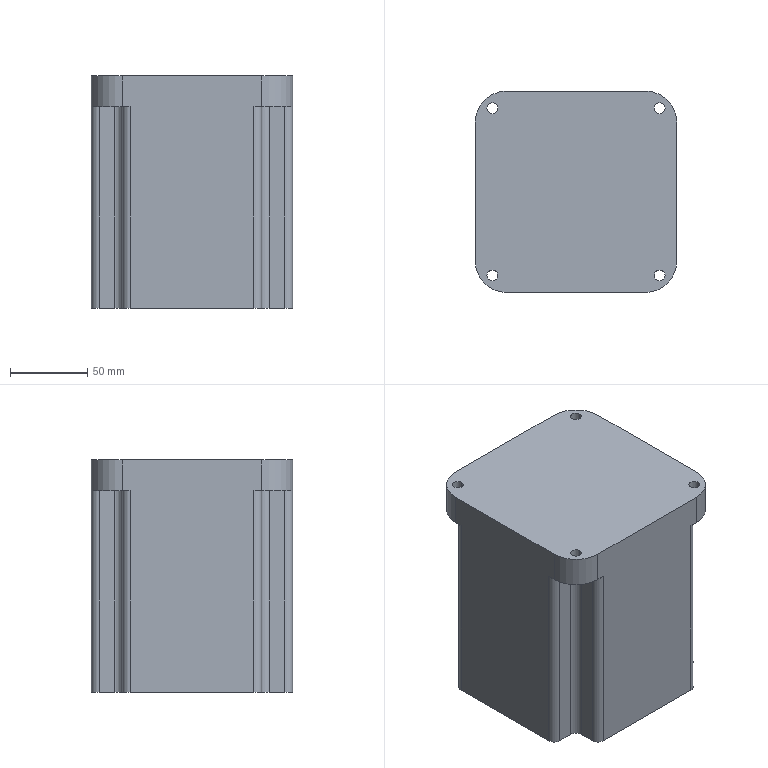Part | SolidWorks | features Fillet 3, CirPattern 2, ICE 2, Extrusion 1, RefAxis 1 | 1 solid | 42 faces | box 130 x 130 x 150 mm | volume 2314264 mm3 | cylinder 24 | plane 18 | commonest cylinder face diameters 10 x12 7 x8 40 x4
STEP:
#1=CARTESIAN_POINT('',(57.5,54.,150.));
#2=VERTEX_POINT('',#1);
#3=CARTESIAN_POINT('',(50.5,54.,150.));
#4=VERTEX_POINT('',#3);
#5=CARTESIAN_POINT('',(54.,54.,150.));
#6=DIRECTION('',(0.,0.,-1.));
#7=DIRECTION('',(-1.,0.,0.));
#8=AXIS2_PLACEMENT_3D('',#5,#6,#7);
#9=CIRCLE('',#8,3.5);
#10=EDGE_CURVE('',#2,#4,#9,.T.);
#11=ORIENTED_EDGE('',*,*,#10,.F.);
#12=CARTESIAN_POINT('',(57.5,54.,130.));
#13=VERTEX_POINT('',#12);
#14=CARTESIAN_POINT('',(57.5,54.,170.));
#15=DIRECTION('',(0.,0.,-1.));
#16=VECTOR('',#15,1000.);
#17=LINE('',#14,#16);
#18=EDGE_CURVE('',#2,#13,#17,.T.);
#19=ORIENTED_EDGE('',*,*,#18,.T.);
#20=CARTESIAN_POINT('',(50.5,54.,130.));
#21=VERTEX_POINT('',#20);
#22=CARTESIAN_POINT('',(54.,54.,130.));
#23=DIRECTION('',(0.,0.,-1.));
#24=DIRECTION('',(0.,1.,0.));
#25=AXIS2_PLACEMENT_3D('',#22,#23,#24);
#26=CIRCLE('',#25,3.5);
#27=EDGE_CURVE('',#13,#21,#26,.T.);
#28=ORIENTED_EDGE('',*,*,#27,.T.);
#29=CARTESIAN_POINT('',(50.5,54.,170.));
#30=DIRECTION('',(0.,0.,-1.));
#31=VECTOR('',#30,1000.);
#32=LINE('',#29,#31);
#33=EDGE_CURVE('',#4,#21,#32,.T.);
#34=ORIENTED_EDGE('',*,*,#33,.F.);
#35=EDGE_LOOP('',(#11,#19,#28,#34));
#36=FACE_OUTER_BOUND('',#35,.T.);
#37=CARTESIAN_POINT('',(54.,54.,170.));
#38=DIRECTION('',(0.,0.,-1.));
#39=DIRECTION('',(-1.,0.,0.));
#40=AXIS2_PLACEMENT_3D('',#37,#38,#39);
#41=CYLINDRICAL_SURFACE('',#40,3.5);
#42=ADVANCED_FACE('',(#36),#41,.F.);
#43=CARTESIAN_POINT('',(57.5,-54.,150.));
#44=VERTEX_POINT('',#43);
#45=CARTESIAN_POINT('',(50.5,-54.,150.));
#46=VERTEX_POINT('',#45);
#47=CARTESIAN_POINT('',(54.,-54.,150.));
#48=DIRECTION('',(0.,0.,-1.));
#49=DIRECTION('',(-1.,0.,0.));
#50=AXIS2_PLACEMENT_3D('',#47,#48,#49);
#51=CIRCLE('',#50,3.5);
#52=EDGE_CURVE('',#44,#46,#51,.T.);
#53=ORIENTED_EDGE('',*,*,#52,.F.);
#54=CARTESIAN_POINT('',(57.5,-54.,130.));
#55=VERTEX_POINT('',#54);
#56=CARTESIAN_POINT('',(57.5,-54.,170.));
#57=DIRECTION('',(0.,0.,-1.));
#58=VECTOR('',#57,1000.);
#59=LINE('',#56,#58);
#60=EDGE_CURVE('',#44,#55,#59,.T.);
#61=ORIENTED_EDGE('',*,*,#60,.T.);
#62=CARTESIAN_POINT('',(50.5,-54.,130.));
#63=VERTEX_POINT('',#62);
#64=CARTESIAN_POINT('',(54.,-54.,130.));
#65=DIRECTION('',(0.,0.,-1.));
#66=DIRECTION('',(1.,0.,0.));
#67=AXIS2_PLACEMENT_3D('',#64,#65,#66);
#68=CIRCLE('',#67,3.5);
#69=EDGE_CURVE('',#55,#63,#68,.T.);
#70=ORIENTED_EDGE('',*,*,#69,.T.);
#71=CARTESIAN_POINT('',(50.5,-54.,170.));
#72=DIRECTION('',(0.,0.,-1.));
#73=VECTOR('',#72,1000.);
#74=LINE('',#71,#73);
#75=EDGE_CURVE('',#46,#63,#74,.T.);
#76=ORIENTED_EDGE('',*,*,#75,.F.);
#77=EDGE_LOOP('',(#53,#61,#70,#76));
#78=FACE_OUTER_BOUND('',#77,.T.);
#79=CARTESIAN_POINT('',(54.,-54.,170.));
#80=DIRECTION('',(0.,0.,-1.));
#81=DIRECTION('',(-1.,0.,0.));
#82=AXIS2_PLACEMENT_3D('',#79,#80,#81);
#83=CYLINDRICAL_SURFACE('',#82,3.5);
#84=ADVANCED_FACE('',(#78),#83,.F.);
#85=CARTESIAN_POINT('',(-50.5,-54.,150.));
#86=VERTEX_POINT('',#85);
#87=CARTESIAN_POINT('',(-57.5,-54.,150.));
#88=VERTEX_POINT('',#87);
#89=CARTESIAN_POINT('',(-54.,-54.,150.));
#90=DIRECTION('',(0.,0.,-1.));
#91=DIRECTION('',(-1.,0.,0.));
#92=AXIS2_PLACEMENT_3D('',#89,#90,#91);
#93=CIRCLE('',#92,3.5);
#94=EDGE_CURVE('',#86,#88,#93,.T.);
#95=ORIENTED_EDGE('',*,*,#94,.F.);
#96=CARTESIAN_POINT('',(-50.5,-54.,130.));
#97=VERTEX_POINT('',#96);
#98=CARTESIAN_POINT('',(-50.5,-54.,170.));
#99=DIRECTION('',(0.,0.,-1.));
#100=VECTOR('',#99,1000.);
#101=LINE('',#98,#100);
#102=EDGE_CURVE('',#86,#97,#101,.T.);
#103=ORIENTED_EDGE('',*,*,#102,.T.);
#104=CARTESIAN_POINT('',(-57.5,-54.,130.));
#105=VERTEX_POINT('',#104);
#106=CARTESIAN_POINT('',(-54.,-54.,130.));
#107=DIRECTION('',(0.,0.,-1.));
#108=DIRECTION('',(0.,-1.,0.));
#109=AXIS2_PLACEMENT_3D('',#106,#107,#108);
#110=CIRCLE('',#109,3.5);
#111=EDGE_CURVE('',#97,#105,#110,.T.);
#112=ORIENTED_EDGE('',*,*,#111,.T.);
#113=CARTESIAN_POINT('',(-57.5,-54.,170.));
#114=DIRECTION('',(0.,0.,-1.));
#115=VECTOR('',#114,1000.);
#116=LINE('',#113,#115);
#117=EDGE_CURVE('',#88,#105,#116,.T.);
#118=ORIENTED_EDGE('',*,*,#117,.F.);
#119=EDGE_LOOP('',(#95,#103,#112,#118));
#120=FACE_OUTER_BOUND('',#119,.T.);
#121=CARTESIAN_POINT('',(-54.,-54.,170.));
#122=DIRECTION('',(0.,0.,-1.));
#123=DIRECTION('',(-1.,0.,0.));
#124=AXIS2_PLACEMENT_3D('',#121,#122,#123);
#125=CYLINDRICAL_SURFACE('',#124,3.5);
#126=ADVANCED_FACE('',(#120),#125,.F.);
#127=CARTESIAN_POINT('',(-50.5,54.,150.));
#128=VERTEX_POINT('',#127);
#129=CARTESIAN_POINT('',(-57.5,54.,150.));
#130=VERTEX_POINT('',#129);
#131=CARTESIAN_POINT('',(-54.,54.,150.));
#132=DIRECTION('',(0.,0.,-1.));
#133=DIRECTION('',(-1.,0.,0.));
#134=AXIS2_PLACEMENT_3D('',#131,#132,#133);
#135=CIRCLE('',#134,3.5);
#136=EDGE_CURVE('',#128,#130,#135,.T.);
#137=ORIENTED_EDGE('',*,*,#136,.F.);
#138=CARTESIAN_POINT('',(-50.5,54.,130.));
#139=VERTEX_POINT('',#138);
#140=CARTESIAN_POINT('',(-50.5,54.,170.));
#141=DIRECTION('',(0.,0.,-1.));
#142=VECTOR('',#141,1000.);
#143=LINE('',#140,#142);
#144=EDGE_CURVE('',#128,#139,#143,.T.);
#145=ORIENTED_EDGE('',*,*,#144,.T.);
#146=CARTESIAN_POINT('',(-57.5,54.,130.));
#147=VERTEX_POINT('',#146);
#148=CARTESIAN_POINT('',(-54.,54.,130.));
#149=DIRECTION('',(0.,0.,-1.));
#150=DIRECTION('',(-1.,0.,0.));
#151=AXIS2_PLACEMENT_3D('',#148,#149,#150);
#152=CIRCLE('',#151,3.5);
#153=EDGE_CURVE('',#139,#147,#152,.T.);
#154=ORIENTED_EDGE('',*,*,#153,.T.);
#155=CARTESIAN_POINT('',(-57.5,54.,170.));
#156=DIRECTION('',(0.,0.,-1.));
#157=VECTOR('',#156,1000.);
#158=LINE('',#155,#157);
#159=EDGE_CURVE('',#130,#147,#158,.T.);
#160=ORIENTED_EDGE('',*,*,#159,.F.);
#161=EDGE_LOOP('',(#137,#145,#154,#160));
#162=FACE_OUTER_BOUND('',#161,.T.);
#163=CARTESIAN_POINT('',(-54.,54.,170.));
#164=DIRECTION('',(0.,0.,-1.));
#165=DIRECTION('',(-1.,0.,0.));
#166=AXIS2_PLACEMENT_3D('',#163,#164,#165);
#167=CYLINDRICAL_SURFACE('',#166,3.5);
#168=ADVANCED_FACE('',(#162),#167,.F.);
#169=CARTESIAN_POINT('',(-65.,-45.,130.));
#170=VERTEX_POINT('',#169);
#171=CARTESIAN_POINT('',(-65.,-45.,150.));
#172=VERTEX_POINT('',#171);
#173=CARTESIAN_POINT('',(-65.,-45.,150.));
#174=DIRECTION('',(0.,0.,1.));
#175=VECTOR('',#174,1000.);
#176=LINE('',#173,#175);
#177=EDGE_CURVE('',#170,#172,#176,.T.);
#178=ORIENTED_EDGE('',*,*,#177,.F.);
#179=CARTESIAN_POINT('',(-45.,-65.,130.));
#180=VERTEX_POINT('',#179);
#181=CARTESIAN_POINT('',(-45.,-45.,130.));
#182=DIRECTION('',(0.,0.,1.));
#183=DIRECTION('',(-1.,0.,0.));
#184=AXIS2_PLACEMENT_3D('',#181,#182,#183);
#185=CIRCLE('',#184,20.);
#186=EDGE_CURVE('',#170,#180,#185,.T.);
#187=ORIENTED_EDGE('',*,*,#186,.T.);
#188=CARTESIAN_POINT('',(-45.,-65.,150.));
#189=VERTEX_POINT('',#188);
#190=CARTESIAN_POINT('',(-45.,-65.,150.));
#191=DIRECTION('',(0.,0.,-1.));
#192=VECTOR('',#191,1000.);
#193=LINE('',#190,#192);
#194=EDGE_CURVE('',#189,#180,#193,.T.);
#195=ORIENTED_EDGE('',*,*,#194,.F.);
#196=CARTESIAN_POINT('',(-45.,-45.,150.));
#197=DIRECTION('',(0.,0.,1.));
#198=DIRECTION('',(-1.,0.,0.));
#199=AXIS2_PLACEMENT_3D('',#196,#197,#198);
#200=CIRCLE('',#199,20.);
#201=EDGE_CURVE('',#172,#189,#200,.T.);
#202=ORIENTED_EDGE('',*,*,#201,.F.);
#203=EDGE_LOOP('',(#178,#187,#195,#202));
#204=FACE_OUTER_BOUND('',#203,.T.);
#205=CARTESIAN_POINT('',(-45.,-45.,150.));
#206=DIRECTION('',(0.,0.,-1.));
#207=DIRECTION('',(-1.,0.,0.));
#208=AXIS2_PLACEMENT_3D('',#205,#206,#207);
#209=CYLINDRICAL_SURFACE('',#208,20.);
#210=ADVANCED_FACE('',(#204),#209,.T.);
#211=CARTESIAN_POINT('',(45.,-65.,130.));
#212=VERTEX_POINT('',#211);
#213=CARTESIAN_POINT('',(45.,-65.,150.));
#214=VERTEX_POINT('',#213);
#215=CARTESIAN_POINT('',(45.,-65.,150.));
#216=DIRECTION('',(0.,0.,1.));
#217=VECTOR('',#216,1000.);
#218=LINE('',#215,#217);
#219=EDGE_CURVE('',#212,#214,#218,.T.);
#220=ORIENTED_EDGE('',*,*,#219,.F.);
#221=CARTESIAN_POINT('',(65.,-45.,130.));
#222=VERTEX_POINT('',#221);
#223=CARTESIAN_POINT('',(45.,-45.,130.));
#224=DIRECTION('',(0.,0.,1.));
#225=DIRECTION('',(-1.,0.,0.));
#226=AXIS2_PLACEMENT_3D('',#223,#224,#225);
#227=CIRCLE('',#226,20.);
#228=EDGE_CURVE('',#212,#222,#227,.T.);
#229=ORIENTED_EDGE('',*,*,#228,.T.);
#230=CARTESIAN_POINT('',(65.,-45.,150.));
#231=VERTEX_POINT('',#230);
#232=CARTESIAN_POINT('',(65.,-45.,150.));
#233=DIRECTION('',(0.,0.,-1.));
#234=VECTOR('',#233,1000.);
#235=LINE('',#232,#234);
#236=EDGE_CURVE('',#231,#222,#235,.T.);
#237=ORIENTED_EDGE('',*,*,#236,.F.);
#238=CARTESIAN_POINT('',(45.,-45.,150.));
#239=DIRECTION('',(0.,0.,1.));
#240=DIRECTION('',(-1.,0.,0.));
#241=AXIS2_PLACEMENT_3D('',#238,#239,#240);
#242=CIRCLE('',#241,20.);
#243=EDGE_CURVE('',#214,#231,#242,.T.);
#244=ORIENTED_EDGE('',*,*,#243,.F.);
#245=EDGE_LOOP('',(#220,#229,#237,#244));
#246=FACE_OUTER_BOUND('',#245,.T.);
#247=CARTESIAN_POINT('',(45.,-45.,150.));
#248=DIRECTION('',(0.,0.,-1.));
#249=DIRECTION('',(-1.,0.,0.));
#250=AXIS2_PLACEMENT_3D('',#247,#248,#249);
#251=CYLINDRICAL_SURFACE('',#250,20.);
#252=ADVANCED_FACE('',(#246),#251,.T.);
#253=CARTESIAN_POINT('',(-45.,65.,130.));
#254=VERTEX_POINT('',#253);
#255=CARTESIAN_POINT('',(-45.,65.,150.));
#256=VERTEX_POINT('',#255);
#257=CARTESIAN_POINT('',(-45.,65.,150.));
#258=DIRECTION('',(0.,0.,1.));
#259=VECTOR('',#258,1000.);
#260=LINE('',#257,#259);
#261=EDGE_CURVE('',#254,#256,#260,.T.);
#262=ORIENTED_EDGE('',*,*,#261,.F.);
#263=CARTESIAN_POINT('',(-65.,45.,130.));
#264=VERTEX_POINT('',#263);
#265=CARTESIAN_POINT('',(-45.,45.,130.));
#266=DIRECTION('',(0.,0.,1.));
#267=DIRECTION('',(-1.,0.,0.));
#268=AXIS2_PLACEMENT_3D('',#265,#266,#267);
#269=CIRCLE('',#268,20.);
#270=EDGE_CURVE('',#254,#264,#269,.T.);
#271=ORIENTED_EDGE('',*,*,#270,.T.);
#272=CARTESIAN_POINT('',(-65.,45.,150.));
#273=VERTEX_POINT('',#272);
#274=CARTESIAN_POINT('',(-65.,45.,150.));
#275=DIRECTION('',(0.,0.,-1.));
#276=VECTOR('',#275,1000.);
#277=LINE('',#274,#276);
#278=EDGE_CURVE('',#273,#264,#277,.T.);
#279=ORIENTED_EDGE('',*,*,#278,.F.);
#280=CARTESIAN_POINT('',(-45.,45.,150.));
#281=DIRECTION('',(0.,0.,1.));
#282=DIRECTION('',(-1.,0.,0.));
#283=AXIS2_PLACEMENT_3D('',#280,#281,#282);
#284=CIRCLE('',#283,20.);
#285=EDGE_CURVE('',#256,#273,#284,.T.);
#286=ORIENTED_EDGE('',*,*,#285,.F.);
#287=EDGE_LOOP('',(#262,#271,#279,#286));
#288=FACE_OUTER_BOUND('',#287,.T.);
#289=CARTESIAN_POINT('',(-45.,45.,150.));
#290=DIRECTION('',(0.,0.,-1.));
#291=DIRECTION('',(-1.,0.,0.));
#292=AXIS2_PLACEMENT_3D('',#289,#290,#291);
#293=CYLINDRICAL_SURFACE('',#292,20.);
#294=ADVANCED_FACE('',(#288),#293,.T.);
#295=CARTESIAN_POINT('',(65.,45.,130.));
#296=VERTEX_POINT('',#295);
#297=CARTESIAN_POINT('',(65.,45.,150.));
#298=VERTEX_POINT('',#297);
#299=CARTESIAN_POINT('',(65.,45.,150.));
#300=DIRECTION('',(0.,0.,1.));
#301=VECTOR('',#300,1000.);
#302=LINE('',#299,#301);
#303=EDGE_CURVE('',#296,#298,#302,.T.);
#304=ORIENTED_EDGE('',*,*,#303,.F.);
#305=CARTESIAN_POINT('',(45.,65.,130.));
#306=VERTEX_POINT('',#305);
#307=CARTESIAN_POINT('',(45.,45.,130.));
#308=DIRECTION('',(0.,0.,1.));
#309=DIRECTION('',(-1.,0.,0.));
#310=AXIS2_PLACEMENT_3D('',#307,#308,#309);
#311=CIRCLE('',#310,20.);
#312=EDGE_CURVE('',#296,#306,#311,.T.);
#313=ORIENTED_EDGE('',*,*,#312,.T.);
#314=CARTESIAN_POINT('',(45.,65.,150.));
#315=VERTEX_POINT('',#314);
#316=CARTESIAN_POINT('',(45.,65.,150.));
#317=DIRECTION('',(0.,0.,-1.));
#318=VECTOR('',#317,1000.);
#319=LINE('',#316,#318);
#320=EDGE_CURVE('',#315,#306,#319,.T.);
#321=ORIENTED_EDGE('',*,*,#320,.F.);
#322=CARTESIAN_POINT('',(45.,45.,150.));
#323=DIRECTION('',(0.,0.,1.));
#324=DIRECTION('',(-1.,0.,0.));
#325=AXIS2_PLACEMENT_3D('',#322,#323,#324);
#326=CIRCLE('',#325,20.);
#327=EDGE_CURVE('',#298,#315,#326,.T.);
#328=ORIENTED_EDGE('',*,*,#327,.F.);
#329=EDGE_LOOP('',(#304,#313,#321,#328));
#330=FACE_OUTER_BOUND('',#329,.T.);
#331=CARTESIAN_POINT('',(45.,45.,150.));
#332=DIRECTION('',(0.,0.,-1.));
#333=DIRECTION('',(-1.,0.,0.));
#334=AXIS2_PLACEMENT_3D('',#331,#332,#333);
#335=CYLINDRICAL_SURFACE('',#334,20.);
#336=ADVANCED_FACE('',(#330),#335,.T.);
#337=CARTESIAN_POINT('',(65.,-40.,0.));
#338=VERTEX_POINT('',#337);
#339=CARTESIAN_POINT('',(65.,40.,0.));
#340=VERTEX_POINT('',#339);
#341=CARTESIAN_POINT('',(65.,-65.,0.));
#342=DIRECTION('',(0.,1.,0.));
#343=VECTOR('',#342,1000.);
#344=LINE('',#341,#343);
#345=EDGE_CURVE('',#338,#340,#344,.T.);
#346=ORIENTED_EDGE('',*,*,#345,.T.);
#347=CARTESIAN_POINT('',(65.,40.,130.));
#348=VERTEX_POINT('',#347);
#349=CARTESIAN_POINT('',(65.,40.,150.));
#350=DIRECTION('',(0.,0.,1.));
#351=VECTOR('',#350,1000.);
#352=LINE('',#349,#351);
#353=EDGE_CURVE('',#340,#348,#352,.T.);
#354=ORIENTED_EDGE('',*,*,#353,.T.);
#355=CARTESIAN_POINT('',(65.,0.,130.));
#356=DIRECTION('',(0.,1.,0.));
#357=VECTOR('',#356,1000.);
#358=LINE('',#355,#357);
#359=EDGE_CURVE('',#348,#296,#358,.T.);
#360=ORIENTED_EDGE('',*,*,#359,.T.);
#361=ORIENTED_EDGE('',*,*,#303,.T.);
#362=CARTESIAN_POINT('',(65.,-65.,150.));
#363=DIRECTION('',(0.,1.,0.));
#364=VECTOR('',#363,1000.);
#365=LINE('',#362,#364);
#366=EDGE_CURVE('',#231,#298,#365,.T.);
#367=ORIENTED_EDGE('',*,*,#366,.F.);
#368=ORIENTED_EDGE('',*,*,#236,.T.);
#369=CARTESIAN_POINT('',(65.,-40.,130.));
#370=VERTEX_POINT('',#369);
#371=CARTESIAN_POINT('',(65.,0.,130.));
#372=DIRECTION('',(0.,1.,0.));
#373=VECTOR('',#372,1000.);
#374=LINE('',#371,#373);
#375=EDGE_CURVE('',#222,#370,#374,.T.);
#376=ORIENTED_EDGE('',*,*,#375,.T.);
#377=CARTESIAN_POINT('',(65.,-40.,150.));
#378=DIRECTION('',(0.,0.,-1.));
#379=VECTOR('',#378,1000.);
#380=LINE('',#377,#379);
#381=EDGE_CURVE('',#370,#338,#380,.T.);
#382=ORIENTED_EDGE('',*,*,#381,.T.);
#383=EDGE_LOOP('',(#346,#354,#360,#361,#367,#368,#376,#382));
#384=FACE_OUTER_BOUND('',#383,.T.);
#385=CARTESIAN_POINT('',(65.,-65.,150.));
#386=DIRECTION('',(-1.,0.,0.));
#387=DIRECTION('',(0.,0.,1.));
#388=AXIS2_PLACEMENT_3D('',#385,#386,#387);
#389=PLANE('',#388);
#390=ADVANCED_FACE('',(#384),#389,.F.);
#391=CARTESIAN_POINT('',(40.,65.,130.));
#392=VERTEX_POINT('',#391);
#393=CARTESIAN_POINT('',(0.,65.,130.));
#394=DIRECTION('',(-1.,0.,0.));
#395=VECTOR('',#394,1000.);
#396=LINE('',#393,#395);
#397=EDGE_CURVE('',#306,#392,#396,.T.);
#398=ORIENTED_EDGE('',*,*,#397,.T.);
#399=CARTESIAN_POINT('',(40.,65.,0.));
#400=VERTEX_POINT('',#399);
#401=CARTESIAN_POINT('',(40.,65.,150.));
#402=DIRECTION('',(0.,0.,-1.));
#403=VECTOR('',#402,1000.);
#404=LINE('',#401,#403);
#405=EDGE_CURVE('',#392,#400,#404,.T.);
#406=ORIENTED_EDGE('',*,*,#405,.T.);
#407=CARTESIAN_POINT('',(-40.,65.,0.));
#408=VERTEX_POINT('',#407);
#409=CARTESIAN_POINT('',(-65.,65.,0.));
#410=DIRECTION('',(-1.,0.,0.));
#411=VECTOR('',#410,1000.);
#412=LINE('',#409,#411);
#413=EDGE_CURVE('',#400,#408,#412,.T.);
#414=ORIENTED_EDGE('',*,*,#413,.T.);
#415=CARTESIAN_POINT('',(-40.,65.,130.));
#416=VERTEX_POINT('',#415);
#417=CARTESIAN_POINT('',(-40.,65.,150.));
#418=DIRECTION('',(0.,0.,1.));
#419=VECTOR('',#418,1000.);
#420=LINE('',#417,#419);
#421=EDGE_CURVE('',#408,#416,#420,.T.);
#422=ORIENTED_EDGE('',*,*,#421,.T.);
#423=CARTESIAN_POINT('',(0.,65.,130.));
#424=DIRECTION('',(-1.,0.,0.));
#425=VECTOR('',#424,1000.);
#426=LINE('',#423,#425);
#427=EDGE_CURVE('',#416,#254,#426,.T.);
#428=ORIENTED_EDGE('',*,*,#427,.T.);
#429=ORIENTED_EDGE('',*,*,#261,.T.);
#430=CARTESIAN_POINT('',(-65.,65.,150.));
#431=DIRECTION('',(-1.,0.,0.));
#432=VECTOR('',#431,1000.);
#433=LINE('',#430,#432);
#434=EDGE_CURVE('',#315,#256,#433,.T.);
#435=ORIENTED_EDGE('',*,*,#434,.F.);
#436=ORIENTED_EDGE('',*,*,#320,.T.);
#437=EDGE_LOOP('',(#398,#406,#414,#422,#428,#429,#435,#436));
#438=FACE_OUTER_BOUND('',#437,.T.);
#439=CARTESIAN_POINT('',(-65.,65.,150.));
#440=DIRECTION('',(0.,-1.,0.));
#441=DIRECTION('',(0.,0.,-1.));
#442=AXIS2_PLACEMENT_3D('',#439,#440,#441);
#443=PLANE('',#442);
#444=ADVANCED_FACE('',(#438),#443,.F.);
#445=CARTESIAN_POINT('',(-65.,40.,130.));
#446=VERTEX_POINT('',#445);
#447=CARTESIAN_POINT('',(-65.,0.,130.));
#448=DIRECTION('',(0.,-1.,0.));
#449=VECTOR('',#448,1000.);
#450=LINE('',#447,#449);
#451=EDGE_CURVE('',#264,#446,#450,.T.);
#452=ORIENTED_EDGE('',*,*,#451,.T.);
#453=CARTESIAN_POINT('',(-65.,40.,0.));
#454=VERTEX_POINT('',#453);
#455=CARTESIAN_POINT('',(-65.,40.,150.));
#456=DIRECTION('',(0.,0.,-1.));
#457=VECTOR('',#456,1000.);
#458=LINE('',#455,#457);
#459=EDGE_CURVE('',#446,#454,#458,.T.);
#460=ORIENTED_EDGE('',*,*,#459,.T.);
#461=CARTESIAN_POINT('',(-65.,-40.,0.));
#462=VERTEX_POINT('',#461);
#463=CARTESIAN_POINT('',(-65.,-65.,0.));
#464=DIRECTION('',(0.,-1.,0.));
#465=VECTOR('',#464,1000.);
#466=LINE('',#463,#465);
#467=EDGE_CURVE('',#454,#462,#466,.T.);
#468=ORIENTED_EDGE('',*,*,#467,.T.);
#469=CARTESIAN_POINT('',(-65.,-40.,130.));
#470=VERTEX_POINT('',#469);
#471=CARTESIAN_POINT('',(-65.,-40.,150.));
#472=DIRECTION('',(0.,0.,1.));
#473=VECTOR('',#472,1000.);
#474=LINE('',#471,#473);
#475=EDGE_CURVE('',#462,#470,#474,.T.);
#476=ORIENTED_EDGE('',*,*,#475,.T.);
#477=CARTESIAN_POINT('',(-65.,0.,130.));
#478=DIRECTION('',(0.,-1.,0.));
#479=VECTOR('',#478,1000.);
#480=LINE('',#477,#479);
#481=EDGE_CURVE('',#470,#170,#480,.T.);
#482=ORIENTED_EDGE('',*,*,#481,.T.);
#483=ORIENTED_EDGE('',*,*,#177,.T.);
#484=CARTESIAN_POINT('',(-65.,-65.,150.));
#485=DIRECTION('',(0.,-1.,0.));
#486=VECTOR('',#485,1000.);
#487=LINE('',#484,#486);
#488=EDGE_CURVE('',#273,#172,#487,.T.);
#489=ORIENTED_EDGE('',*,*,#488,.F.);
#490=ORIENTED_EDGE('',*,*,#278,.T.);
#491=EDGE_LOOP('',(#452,#460,#468,#476,#482,#483,#489,#490));
#492=FACE_OUTER_BOUND('',#491,.T.);
#493=CARTESIAN_POINT('',(-65.,-65.,150.));
#494=DIRECTION('',(1.,0.,0.));
#495=DIRECTION('',(0.,0.,-1.));
#496=AXIS2_PLACEMENT_3D('',#493,#494,#495);
#497=PLANE('',#496);
#498=ADVANCED_FACE('',(#492),#497,.F.);
#499=CARTESIAN_POINT('',(-40.,-65.,130.));
#500=VERTEX_POINT('',#499);
#501=CARTESIAN_POINT('',(0.,-65.,130.));
#502=DIRECTION('',(1.,0.,0.));
#503=VECTOR('',#502,1000.);
#504=LINE('',#501,#503);
#505=EDGE_CURVE('',#180,#500,#504,.T.);
#506=ORIENTED_EDGE('',*,*,#505,.T.);
#507=CARTESIAN_POINT('',(-40.,-65.,0.));
#508=VERTEX_POINT('',#507);
#509=CARTESIAN_POINT('',(-40.,-65.,150.));
#510=DIRECTION('',(0.,0.,-1.));
#511=VECTOR('',#510,1000.);
#512=LINE('',#509,#511);
#513=EDGE_CURVE('',#500,#508,#512,.T.);
#514=ORIENTED_EDGE('',*,*,#513,.T.);
#515=CARTESIAN_POINT('',(40.,-65.,0.));
#516=VERTEX_POINT('',#515);
#517=CARTESIAN_POINT('',(-65.,-65.,0.));
#518=DIRECTION('',(1.,0.,0.));
#519=VECTOR('',#518,1000.);
#520=LINE('',#517,#519);
#521=EDGE_CURVE('',#508,#516,#520,.T.);
#522=ORIENTED_EDGE('',*,*,#521,.T.);
#523=CARTESIAN_POINT('',(40.,-65.,130.));
#524=VERTEX_POINT('',#523);
#525=CARTESIAN_POINT('',(40.,-65.,150.));
#526=DIRECTION('',(0.,0.,1.));
#527=VECTOR('',#526,1000.);
#528=LINE('',#525,#527);
#529=EDGE_CURVE('',#516,#524,#528,.T.);
#530=ORIENTED_EDGE('',*,*,#529,.T.);
#531=CARTESIAN_POINT('',(0.,-65.,130.));
#532=DIRECTION('',(1.,0.,0.));
#533=VECTOR('',#532,1000.);
#534=LINE('',#531,#533);
#535=EDGE_CURVE('',#524,#212,#534,.T.);
#536=ORIENTED_EDGE('',*,*,#535,.T.);
#537=ORIENTED_EDGE('',*,*,#219,.T.);
#538=CARTESIAN_POINT('',(-65.,-65.,150.));
#539=DIRECTION('',(1.,0.,0.));
#540=VECTOR('',#539,1000.);
#541=LINE('',#538,#540);
#542=EDGE_CURVE('',#189,#214,#541,.T.);
#543=ORIENTED_EDGE('',*,*,#542,.F.);
#544=ORIENTED_EDGE('',*,*,#194,.T.);
#545=EDGE_LOOP('',(#506,#514,#522,#530,#536,#537,#543,#544));
#546=FACE_OUTER_BOUND('',#545,.T.);
#547=CARTESIAN_POINT('',(-65.,-65.,150.));
#548=DIRECTION('',(0.,1.,0.));
#549=DIRECTION('',(0.,0.,1.));
#550=AXIS2_PLACEMENT_3D('',#547,#548,#549);
#551=PLANE('',#550);
#552=ADVANCED_FACE('',(#546),#551,.F.);
#553=CARTESIAN_POINT('',(-54.,-54.,150.));
#554=DIRECTION('',(0.,0.,-1.));
#555=DIRECTION('',(-1.,0.,0.));
#556=AXIS2_PLACEMENT_3D('',#553,#554,#555);
#557=CIRCLE('',#556,3.5);
#558=EDGE_CURVE('',#88,#86,#557,.T.);
#559=ORIENTED_EDGE('',*,*,#558,.T.);
#560=ORIENTED_EDGE('',*,*,#94,.T.);
#561=EDGE_LOOP('',(#559,#560));
#562=FACE_BOUND('',#561,.T.);
#563=CARTESIAN_POINT('',(54.,-54.,150.));
#564=DIRECTION('',(0.,0.,-1.));
#565=DIRECTION('',(-1.,0.,0.));
#566=AXIS2_PLACEMENT_3D('',#563,#564,#565);
#567=CIRCLE('',#566,3.5);
#568=EDGE_CURVE('',#46,#44,#567,.T.);
#569=ORIENTED_EDGE('',*,*,#568,.T.);
#570=ORIENTED_EDGE('',*,*,#52,.T.);
#571=EDGE_LOOP('',(#569,#570));
#572=FACE_BOUND('',#571,.T.);
#573=CARTESIAN_POINT('',(54.,54.,150.));
#574=DIRECTION('',(0.,0.,-1.));
#575=DIRECTION('',(-1.,0.,0.));
#576=AXIS2_PLACEMENT_3D('',#573,#574,#575);
#577=CIRCLE('',#576,3.5);
#578=EDGE_CURVE('',#4,#2,#577,.T.);
#579=ORIENTED_EDGE('',*,*,#578,.T.);
#580=ORIENTED_EDGE('',*,*,#10,.T.);
#581=EDGE_LOOP('',(#579,#580));
#582=FACE_BOUND('',#581,.T.);
#583=CARTESIAN_POINT('',(-54.,54.,150.));
#584=DIRECTION('',(0.,0.,-1.));
#585=DIRECTION('',(-1.,0.,0.));
#586=AXIS2_PLACEMENT_3D('',#583,#584,#585);
#587=CIRCLE('',#586,3.5);
#588=EDGE_CURVE('',#130,#128,#587,.T.);
#589=ORIENTED_EDGE('',*,*,#588,.T.);
#590=ORIENTED_EDGE('',*,*,#136,.T.);
#591=EDGE_LOOP('',(#589,#590));
#592=FACE_BOUND('',#591,.T.);
#593=ORIENTED_EDGE('',*,*,#488,.T.);
#594=ORIENTED_EDGE('',*,*,#201,.T.);
#595=ORIENTED_EDGE('',*,*,#542,.T.);
#596=ORIENTED_EDGE('',*,*,#243,.T.);
#597=ORIENTED_EDGE('',*,*,#366,.T.);
#598=ORIENTED_EDGE('',*,*,#327,.T.);
#599=ORIENTED_EDGE('',*,*,#434,.T.);
#600=ORIENTED_EDGE('',*,*,#285,.T.);
#601=EDGE_LOOP('',(#593,#594,#595,#596,#597,#598,#599,#600));
#602=FACE_OUTER_BOUND('',#601,.T.);
#603=CARTESIAN_POINT('',(0.,0.,150.));
#604=DIRECTION('',(0.,0.,-1.));
#605=DIRECTION('',(-1.,0.,0.));
#606=AXIS2_PLACEMENT_3D('',#603,#604,#605);
#607=PLANE('',#606);
#608=ADVANCED_FACE('',(#562,#572,#582,#592,#602),#607,.F.);
#609=CARTESIAN_POINT('',(60.,45.,0.));
#610=VERTEX_POINT('',#609);
#611=CARTESIAN_POINT('',(50.,45.,0.));
#612=VERTEX_POINT('',#611);
#613=CARTESIAN_POINT('',(114.063,45.,0.));
#614=DIRECTION('',(-1.,0.,0.));
#615=VECTOR('',#614,1000.);
#616=LINE('',#613,#615);
#617=EDGE_CURVE('',#610,#612,#616,.T.);
#618=ORIENTED_EDGE('',*,*,#617,.F.);
#619=CARTESIAN_POINT('',(60.,40.,0.));
#620=DIRECTION('',(0.,0.,-1.));
#621=DIRECTION('',(-1.,0.,0.));
#622=AXIS2_PLACEMENT_3D('',#619,#620,#621);
#623=CIRCLE('',#622,5.);
#624=EDGE_CURVE('',#610,#340,#623,.T.);
#625=ORIENTED_EDGE('',*,*,#624,.T.);
#626=ORIENTED_EDGE('',*,*,#345,.F.);
#627=CARTESIAN_POINT('',(60.,-45.,0.));
#628=VERTEX_POINT('',#627);
#629=CARTESIAN_POINT('',(60.,-40.,0.));
#630=DIRECTION('',(0.,0.,-1.));
#631=DIRECTION('',(-1.,0.,0.));
#632=AXIS2_PLACEMENT_3D('',#629,#630,#631);
#633=CIRCLE('',#632,5.);
#634=EDGE_CURVE('',#338,#628,#633,.T.);
#635=ORIENTED_EDGE('',*,*,#634,.T.);
#636=CARTESIAN_POINT('',(50.,-45.,0.));
#637=VERTEX_POINT('',#636);
#638=CARTESIAN_POINT('',(130.712,-45.,0.));
#639=DIRECTION('',(1.,0.,0.));
#640=VECTOR('',#639,1000.);
#641=LINE('',#638,#640);
#642=EDGE_CURVE('',#637,#628,#641,.T.);
#643=ORIENTED_EDGE('',*,*,#642,.F.);
#644=CARTESIAN_POINT('',(45.,-50.,0.));
#645=VERTEX_POINT('',#644);
#646=CARTESIAN_POINT('',(50.,-50.,0.));
#647=DIRECTION('',(0.,0.,1.));
#648=DIRECTION('',(-1.,0.,0.));
#649=AXIS2_PLACEMENT_3D('',#646,#647,#648);
#650=CIRCLE('',#649,5.);
#651=EDGE_CURVE('',#637,#645,#650,.T.);
#652=ORIENTED_EDGE('',*,*,#651,.T.);
#653=CARTESIAN_POINT('',(45.,-60.,0.));
#654=VERTEX_POINT('',#653);
#655=CARTESIAN_POINT('',(45.,-114.063,0.));
#656=DIRECTION('',(0.,1.,0.));
#657=VECTOR('',#656,1000.);
#658=LINE('',#655,#657);
#659=EDGE_CURVE('',#654,#645,#658,.T.);
#660=ORIENTED_EDGE('',*,*,#659,.F.);
#661=CARTESIAN_POINT('',(40.,-60.,0.));
#662=DIRECTION('',(0.,0.,-1.));
#663=DIRECTION('',(-1.,0.,0.));
#664=AXIS2_PLACEMENT_3D('',#661,#662,#663);
#665=CIRCLE('',#664,5.);
#666=EDGE_CURVE('',#654,#516,#665,.T.);
#667=ORIENTED_EDGE('',*,*,#666,.T.);
#668=ORIENTED_EDGE('',*,*,#521,.F.);
#669=CARTESIAN_POINT('',(-45.,-60.,0.));
#670=VERTEX_POINT('',#669);
#671=CARTESIAN_POINT('',(-40.,-60.,0.));
#672=DIRECTION('',(0.,0.,-1.));
#673=DIRECTION('',(-1.,0.,0.));
#674=AXIS2_PLACEMENT_3D('',#671,#672,#673);
#675=CIRCLE('',#674,5.);
#676=EDGE_CURVE('',#508,#670,#675,.T.);
#677=ORIENTED_EDGE('',*,*,#676,.T.);
#678=CARTESIAN_POINT('',(-45.,-50.,0.));
#679=VERTEX_POINT('',#678);
#680=CARTESIAN_POINT('',(-45.,-130.712,0.));
#681=DIRECTION('',(0.,-1.,0.));
#682=VECTOR('',#681,1000.);
#683=LINE('',#680,#682);
#684=EDGE_CURVE('',#679,#670,#683,.T.);
#685=ORIENTED_EDGE('',*,*,#684,.F.);
#686=CARTESIAN_POINT('',(-50.,-45.,0.));
#687=VERTEX_POINT('',#686);
#688=CARTESIAN_POINT('',(-50.,-50.,0.));
#689=DIRECTION('',(0.,0.,1.));
#690=DIRECTION('',(-1.,0.,0.));
#691=AXIS2_PLACEMENT_3D('',#688,#689,#690);
#692=CIRCLE('',#691,5.);
#693=EDGE_CURVE('',#679,#687,#692,.T.);
#694=ORIENTED_EDGE('',*,*,#693,.T.);
#695=CARTESIAN_POINT('',(-60.,-45.,0.));
#696=VERTEX_POINT('',#695);
#697=CARTESIAN_POINT('',(-114.063,-45.,0.));
#698=DIRECTION('',(1.,0.,0.));
#699=VECTOR('',#698,1000.);
#700=LINE('',#697,#699);
#701=EDGE_CURVE('',#696,#687,#700,.T.);
#702=ORIENTED_EDGE('',*,*,#701,.F.);
#703=CARTESIAN_POINT('',(-60.,-40.,0.));
#704=DIRECTION('',(0.,0.,-1.));
#705=DIRECTION('',(-1.,0.,0.));
#706=AXIS2_PLACEMENT_3D('',#703,#704,#705);
#707=CIRCLE('',#706,5.);
#708=EDGE_CURVE('',#696,#462,#707,.T.);
#709=ORIENTED_EDGE('',*,*,#708,.T.);
#710=ORIENTED_EDGE('',*,*,#467,.F.);
#711=CARTESIAN_POINT('',(-60.,45.,0.));
#712=VERTEX_POINT('',#711);
#713=CARTESIAN_POINT('',(-60.,40.,0.));
#714=DIRECTION('',(0.,0.,-1.));
#715=DIRECTION('',(-1.,0.,0.));
#716=AXIS2_PLACEMENT_3D('',#713,#714,#715);
#717=CIRCLE('',#716,5.);
#718=EDGE_CURVE('',#454,#712,#717,.T.);
#719=ORIENTED_EDGE('',*,*,#718,.T.);
#720=CARTESIAN_POINT('',(-50.,45.,0.));
#721=VERTEX_POINT('',#720);
#722=CARTESIAN_POINT('',(-130.712,45.,0.));
#723=DIRECTION('',(-1.,0.,0.));
#724=VECTOR('',#723,1000.);
#725=LINE('',#722,#724);
#726=EDGE_CURVE('',#721,#712,#725,.T.);
#727=ORIENTED_EDGE('',*,*,#726,.F.);
#728=CARTESIAN_POINT('',(-45.,50.,0.));
#729=VERTEX_POINT('',#728);
#730=CARTESIAN_POINT('',(-50.,50.,0.));
#731=DIRECTION('',(0.,0.,1.));
#732=DIRECTION('',(-1.,0.,0.));
#733=AXIS2_PLACEMENT_3D('',#730,#731,#732);
#734=CIRCLE('',#733,5.);
#735=EDGE_CURVE('',#721,#729,#734,.T.);
#736=ORIENTED_EDGE('',*,*,#735,.T.);
#737=CARTESIAN_POINT('',(-45.,60.,0.));
#738=VERTEX_POINT('',#737);
#739=CARTESIAN_POINT('',(-45.,114.063,0.));
#740=DIRECTION('',(0.,-1.,0.));
#741=VECTOR('',#740,1000.);
#742=LINE('',#739,#741);
#743=EDGE_CURVE('',#738,#729,#742,.T.);
#744=ORIENTED_EDGE('',*,*,#743,.F.);
#745=CARTESIAN_POINT('',(-40.,60.,0.));
#746=DIRECTION('',(0.,0.,-1.));
#747=DIRECTION('',(-1.,0.,0.));
#748=AXIS2_PLACEMENT_3D('',#745,#746,#747);
#749=CIRCLE('',#748,5.);
#750=EDGE_CURVE('',#738,#408,#749,.T.);
#751=ORIENTED_EDGE('',*,*,#750,.T.);
#752=ORIENTED_EDGE('',*,*,#413,.F.);
#753=CARTESIAN_POINT('',(45.,60.,0.));
#754=VERTEX_POINT('',#753);
#755=CARTESIAN_POINT('',(40.,60.,0.));
#756=DIRECTION('',(0.,0.,-1.));
#757=DIRECTION('',(-1.,0.,0.));
#758=AXIS2_PLACEMENT_3D('',#755,#756,#757);
#759=CIRCLE('',#758,5.);
#760=EDGE_CURVE('',#400,#754,#759,.T.);
#761=ORIENTED_EDGE('',*,*,#760,.T.);
#762=CARTESIAN_POINT('',(45.,50.,0.));
#763=VERTEX_POINT('',#762);
#764=CARTESIAN_POINT('',(45.,130.712,0.));
#765=DIRECTION('',(0.,1.,0.));
#766=VECTOR('',#765,1000.);
#767=LINE('',#764,#766);
#768=EDGE_CURVE('',#763,#754,#767,.T.);
#769=ORIENTED_EDGE('',*,*,#768,.F.);
#770=CARTESIAN_POINT('',(50.,50.,0.));
#771=DIRECTION('',(0.,0.,1.));
#772=DIRECTION('',(-1.,0.,0.));
#773=AXIS2_PLACEMENT_3D('',#770,#771,#772);
#774=CIRCLE('',#773,5.);
#775=EDGE_CURVE('',#763,#612,#774,.T.);
#776=ORIENTED_EDGE('',*,*,#775,.T.);
#777=EDGE_LOOP('',(#618,#625,#626,#635,#643,#652,#660,#667,#668,#677,#685,#694,#702,#709,#710,#719,#727,#736,#744,#751,#752,#761,#769,#776));
#778=FACE_OUTER_BOUND('',#777,.T.);
#779=CARTESIAN_POINT('',(0.,0.,0.));
#780=DIRECTION('',(0.,0.,-1.));
#781=DIRECTION('',(-1.,0.,0.));
#782=AXIS2_PLACEMENT_3D('',#779,#780,#781);
#783=PLANE('',#782);
#784=ADVANCED_FACE('',(#778),#783,.T.);
#785=ORIENTED_EDGE('',*,*,#768,.T.);
#786=CARTESIAN_POINT('',(45.,60.,130.));
#787=VERTEX_POINT('',#786);
#788=CARTESIAN_POINT('',(45.,60.,130.));
#789=DIRECTION('',(0.,0.,1.));
#790=VECTOR('',#789,1000.);
#791=LINE('',#788,#790);
#792=EDGE_CURVE('',#754,#787,#791,.T.);
#793=ORIENTED_EDGE('',*,*,#792,.T.);
#794=CARTESIAN_POINT('',(45.,50.,130.));
#795=VERTEX_POINT('',#794);
#796=CARTESIAN_POINT('',(45.,130.712,130.));
#797=DIRECTION('',(0.,1.,0.));
#798=VECTOR('',#797,1000.);
#799=LINE('',#796,#798);
#800=EDGE_CURVE('',#795,#787,#799,.T.);
#801=ORIENTED_EDGE('',*,*,#800,.F.);
#802=CARTESIAN_POINT('',(45.,50.,0.));
#803=DIRECTION('',(0.,0.,-1.));
#804=VECTOR('',#803,1000.);
#805=LINE('',#802,#804);
#806=EDGE_CURVE('',#795,#763,#805,.T.);
#807=ORIENTED_EDGE('',*,*,#806,.T.);
#808=EDGE_LOOP('',(#785,#793,#801,#807));
#809=FACE_OUTER_BOUND('',#808,.T.);
#810=CARTESIAN_POINT('',(45.,130.712,130.));
#811=DIRECTION('',(-1.,0.,0.));
#812=DIRECTION('',(0.,0.,1.));
#813=AXIS2_PLACEMENT_3D('',#810,#811,#812);
#814=PLANE('',#813);
#815=ADVANCED_FACE('',(#809),#814,.F.);
#816=CARTESIAN_POINT('',(60.,45.,130.));
#817=VERTEX_POINT('',#816);
#818=CARTESIAN_POINT('',(50.,45.,130.));
#819=VERTEX_POINT('',#818);
#820=CARTESIAN_POINT('',(114.063,45.,130.));
#821=DIRECTION('',(-1.,0.,0.));
#822=VECTOR('',#821,1000.);
#823=LINE('',#820,#822);
#824=EDGE_CURVE('',#817,#819,#823,.T.);
#825=ORIENTED_EDGE('',*,*,#824,.F.);
#826=CARTESIAN_POINT('',(60.,45.,130.));
#827=DIRECTION('',(0.,0.,-1.));
#828=VECTOR('',#827,1000.);
#829=LINE('',#826,#828);
#830=EDGE_CURVE('',#817,#610,#829,.T.);
#831=ORIENTED_EDGE('',*,*,#830,.T.);
#832=ORIENTED_EDGE('',*,*,#617,.T.);
#833=CARTESIAN_POINT('',(50.,45.,130.));
#834=DIRECTION('',(0.,0.,1.));
#835=VECTOR('',#834,1000.);
#836=LINE('',#833,#835);
#837=EDGE_CURVE('',#612,#819,#836,.T.);
#838=ORIENTED_EDGE('',*,*,#837,.T.);
#839=EDGE_LOOP('',(#825,#831,#832,#838));
#840=FACE_OUTER_BOUND('',#839,.T.);
#841=CARTESIAN_POINT('',(114.063,45.,130.));
#842=DIRECTION('',(0.,-1.,0.));
#843=DIRECTION('',(0.,0.,-1.));
#844=AXIS2_PLACEMENT_3D('',#841,#842,#843);
#845=PLANE('',#844);
#846=ADVANCED_FACE('',(#840),#845,.F.);
#847=CARTESIAN_POINT('',(54.,54.,130.));
#848=DIRECTION('',(0.,0.,-1.));
#849=DIRECTION('',(0.,1.,0.));
#850=AXIS2_PLACEMENT_3D('',#847,#848,#849);
#851=CIRCLE('',#850,3.5);
#852=EDGE_CURVE('',#21,#13,#851,.T.);
#853=ORIENTED_EDGE('',*,*,#852,.F.);
#854=ORIENTED_EDGE('',*,*,#27,.F.);
#855=EDGE_LOOP('',(#853,#854));
#856=FACE_BOUND('',#855,.T.);
#857=ORIENTED_EDGE('',*,*,#312,.F.);
#858=ORIENTED_EDGE('',*,*,#359,.F.);
#859=CARTESIAN_POINT('',(60.,40.,130.));
#860=DIRECTION('',(0.,0.,1.));
#861=DIRECTION('',(-1.,0.,0.));
#862=AXIS2_PLACEMENT_3D('',#859,#860,#861);
#863=CIRCLE('',#862,5.);
#864=EDGE_CURVE('',#348,#817,#863,.T.);
#865=ORIENTED_EDGE('',*,*,#864,.T.);
#866=ORIENTED_EDGE('',*,*,#824,.T.);
#867=CARTESIAN_POINT('',(50.,50.,130.));
#868=DIRECTION('',(0.,0.,-1.));
#869=DIRECTION('',(-1.,0.,0.));
#870=AXIS2_PLACEMENT_3D('',#867,#868,#869);
#871=CIRCLE('',#870,5.);
#872=EDGE_CURVE('',#819,#795,#871,.T.);
#873=ORIENTED_EDGE('',*,*,#872,.T.);
#874=ORIENTED_EDGE('',*,*,#800,.T.);
#875=CARTESIAN_POINT('',(40.,60.,130.));
#876=DIRECTION('',(0.,0.,1.));
#877=DIRECTION('',(-1.,0.,0.));
#878=AXIS2_PLACEMENT_3D('',#875,#876,#877);
#879=CIRCLE('',#878,5.);
#880=EDGE_CURVE('',#787,#392,#879,.T.);
#881=ORIENTED_EDGE('',*,*,#880,.T.);
#882=ORIENTED_EDGE('',*,*,#397,.F.);
#883=EDGE_LOOP('',(#857,#858,#865,#866,#873,#874,#881,#882));
#884=FACE_OUTER_BOUND('',#883,.T.);
#885=CARTESIAN_POINT('',(0.,0.,130.));
#886=DIRECTION('',(0.,0.,-1.));
#887=DIRECTION('',(-1.,0.,0.));
#888=AXIS2_PLACEMENT_3D('',#885,#886,#887);
#889=PLANE('',#888);
#890=ADVANCED_FACE('',(#856,#884),#889,.T.);
#891=ORIENTED_EDGE('',*,*,#726,.T.);
#892=CARTESIAN_POINT('',(-60.,45.,130.));
#893=VERTEX_POINT('',#892);
#894=CARTESIAN_POINT('',(-60.,45.,130.));
#895=DIRECTION('',(0.,0.,1.));
#896=VECTOR('',#895,1000.);
#897=LINE('',#894,#896);
#898=EDGE_CURVE('',#712,#893,#897,.T.);
#899=ORIENTED_EDGE('',*,*,#898,.T.);
#900=CARTESIAN_POINT('',(-50.,45.,130.));
#901=VERTEX_POINT('',#900);
#902=CARTESIAN_POINT('',(-130.712,45.,130.));
#903=DIRECTION('',(-1.,0.,0.));
#904=VECTOR('',#903,1000.);
#905=LINE('',#902,#904);
#906=EDGE_CURVE('',#901,#893,#905,.T.);
#907=ORIENTED_EDGE('',*,*,#906,.F.);
#908=CARTESIAN_POINT('',(-50.,45.,0.));
#909=DIRECTION('',(0.,0.,-1.));
#910=VECTOR('',#909,1000.);
#911=LINE('',#908,#910);
#912=EDGE_CURVE('',#901,#721,#911,.T.);
#913=ORIENTED_EDGE('',*,*,#912,.T.);
#914=EDGE_LOOP('',(#891,#899,#907,#913));
#915=FACE_OUTER_BOUND('',#914,.T.);
#916=CARTESIAN_POINT('',(-130.712,45.,130.));
#917=DIRECTION('',(0.,-1.,0.));
#918=DIRECTION('',(1.,0.,0.));
#919=AXIS2_PLACEMENT_3D('',#916,#917,#918);
#920=PLANE('',#919);
#921=ADVANCED_FACE('',(#915),#920,.F.);
#922=CARTESIAN_POINT('',(-45.,60.,130.));
#923=VERTEX_POINT('',#922);
#924=CARTESIAN_POINT('',(-45.,50.,130.));
#925=VERTEX_POINT('',#924);
#926=CARTESIAN_POINT('',(-45.,114.063,130.));
#927=DIRECTION('',(0.,-1.,0.));
#928=VECTOR('',#927,1000.);
#929=LINE('',#926,#928);
#930=EDGE_CURVE('',#923,#925,#929,.T.);
#931=ORIENTED_EDGE('',*,*,#930,.F.);
#932=CARTESIAN_POINT('',(-45.,60.,130.));
#933=DIRECTION('',(0.,0.,-1.));
#934=VECTOR('',#933,1000.);
#935=LINE('',#932,#934);
#936=EDGE_CURVE('',#923,#738,#935,.T.);
#937=ORIENTED_EDGE('',*,*,#936,.T.);
#938=ORIENTED_EDGE('',*,*,#743,.T.);
#939=CARTESIAN_POINT('',(-45.,50.,130.));
#940=DIRECTION('',(0.,0.,1.));
#941=VECTOR('',#940,1000.);
#942=LINE('',#939,#941);
#943=EDGE_CURVE('',#729,#925,#942,.T.);
#944=ORIENTED_EDGE('',*,*,#943,.T.);
#945=EDGE_LOOP('',(#931,#937,#938,#944));
#946=FACE_OUTER_BOUND('',#945,.T.);
#947=CARTESIAN_POINT('',(-45.,114.063,130.));
#948=DIRECTION('',(1.,0.,0.));
#949=DIRECTION('',(0.,1.,0.));
#950=AXIS2_PLACEMENT_3D('',#947,#948,#949);
#951=PLANE('',#950);
#952=ADVANCED_FACE('',(#946),#951,.F.);
#953=CARTESIAN_POINT('',(-54.,54.,130.));
#954=DIRECTION('',(0.,0.,-1.));
#955=DIRECTION('',(-1.,0.,0.));
#956=AXIS2_PLACEMENT_3D('',#953,#954,#955);
#957=CIRCLE('',#956,3.5);
#958=EDGE_CURVE('',#147,#139,#957,.T.);
#959=ORIENTED_EDGE('',*,*,#958,.F.);
#960=ORIENTED_EDGE('',*,*,#153,.F.);
#961=EDGE_LOOP('',(#959,#960));
#962=FACE_BOUND('',#961,.T.);
#963=ORIENTED_EDGE('',*,*,#270,.F.);
#964=ORIENTED_EDGE('',*,*,#427,.F.);
#965=CARTESIAN_POINT('',(-40.,60.,130.));
#966=DIRECTION('',(0.,0.,1.));
#967=DIRECTION('',(-1.,0.,0.));
#968=AXIS2_PLACEMENT_3D('',#965,#966,#967);
#969=CIRCLE('',#968,5.);
#970=EDGE_CURVE('',#416,#923,#969,.T.);
#971=ORIENTED_EDGE('',*,*,#970,.T.);
#972=ORIENTED_EDGE('',*,*,#930,.T.);
#973=CARTESIAN_POINT('',(-50.,50.,130.));
#974=DIRECTION('',(0.,0.,-1.));
#975=DIRECTION('',(-1.,0.,0.));
#976=AXIS2_PLACEMENT_3D('',#973,#974,#975);
#977=CIRCLE('',#976,5.);
#978=EDGE_CURVE('',#925,#901,#977,.T.);
#979=ORIENTED_EDGE('',*,*,#978,.T.);
#980=ORIENTED_EDGE('',*,*,#906,.T.);
#981=CARTESIAN_POINT('',(-60.,40.,130.));
#982=DIRECTION('',(0.,0.,1.));
#983=DIRECTION('',(-1.,0.,0.));
#984=AXIS2_PLACEMENT_3D('',#981,#982,#983);
#985=CIRCLE('',#984,5.);
#986=EDGE_CURVE('',#893,#446,#985,.T.);
#987=ORIENTED_EDGE('',*,*,#986,.T.);
#988=ORIENTED_EDGE('',*,*,#451,.F.);
#989=EDGE_LOOP('',(#963,#964,#971,#972,#979,#980,#987,#988));
#990=FACE_OUTER_BOUND('',#989,.T.);
#991=CARTESIAN_POINT('',(0.,0.,130.));
#992=DIRECTION('',(0.,0.,-1.));
#993=DIRECTION('',(0.,-1.,0.));
#994=AXIS2_PLACEMENT_3D('',#991,#992,#993);
#995=PLANE('',#994);
#996=ADVANCED_FACE('',(#962,#990),#995,.T.);
#997=ORIENTED_EDGE('',*,*,#642,.T.);
#998=CARTESIAN_POINT('',(60.,-45.,130.));
#999=VERTEX_POINT('',#998);
#1000=CARTESIAN_POINT('',(60.,-45.,130.));
#1001=DIRECTION('',(0.,0.,1.));
#1002=VECTOR('',#1001,1000.);
#1003=LINE('',#1000,#1002);
#1004=EDGE_CURVE('',#628,#999,#1003,.T.);
#1005=ORIENTED_EDGE('',*,*,#1004,.T.);
#1006=CARTESIAN_POINT('',(50.,-45.,130.));
#1007=VERTEX_POINT('',#1006);
#1008=CARTESIAN_POINT('',(130.712,-45.,130.));
#1009=DIRECTION('',(1.,0.,0.));
#1010=VECTOR('',#1009,1000.);
#1011=LINE('',#1008,#1010);
#1012=EDGE_CURVE('',#1007,#999,#1011,.T.);
#1013=ORIENTED_EDGE('',*,*,#1012,.F.);
#1014=CARTESIAN_POINT('',(50.,-45.,0.));
#1015=DIRECTION('',(0.,0.,-1.));
#1016=VECTOR('',#1015,1000.);
#1017=LINE('',#1014,#1016);
#1018=EDGE_CURVE('',#1007,#637,#1017,.T.);
#1019=ORIENTED_EDGE('',*,*,#1018,.T.);
#1020=EDGE_LOOP('',(#997,#1005,#1013,#1019));
#1021=FACE_OUTER_BOUND('',#1020,.T.);
#1022=CARTESIAN_POINT('',(130.712,-45.,130.));
#1023=DIRECTION('',(0.,1.,0.));
#1024=DIRECTION('',(-1.,0.,0.));
#1025=AXIS2_PLACEMENT_3D('',#1022,#1023,#1024);
#1026=PLANE('',#1025);
#1027=ADVANCED_FACE('',(#1021),#1026,.F.);
#1028=CARTESIAN_POINT('',(45.,-60.,130.));
#1029=VERTEX_POINT('',#1028);
#1030=CARTESIAN_POINT('',(45.,-50.,130.));
#1031=VERTEX_POINT('',#1030);
#1032=CARTESIAN_POINT('',(45.,-114.063,130.));
#1033=DIRECTION('',(0.,1.,0.));
#1034=VECTOR('',#1033,1000.);
#1035=LINE('',#1032,#1034);
#1036=EDGE_CURVE('',#1029,#1031,#1035,.T.);
#1037=ORIENTED_EDGE('',*,*,#1036,.F.);
#1038=CARTESIAN_POINT('',(45.,-60.,130.));
#1039=DIRECTION('',(0.,0.,-1.));
#1040=VECTOR('',#1039,1000.);
#1041=LINE('',#1038,#1040);
#1042=EDGE_CURVE('',#1029,#654,#1041,.T.);
#1043=ORIENTED_EDGE('',*,*,#1042,.T.);
#1044=ORIENTED_EDGE('',*,*,#659,.T.);
#1045=CARTESIAN_POINT('',(45.,-50.,130.));
#1046=DIRECTION('',(0.,0.,1.));
#1047=VECTOR('',#1046,1000.);
#1048=LINE('',#1045,#1047);
#1049=EDGE_CURVE('',#645,#1031,#1048,.T.);
#1050=ORIENTED_EDGE('',*,*,#1049,.T.);
#1051=EDGE_LOOP('',(#1037,#1043,#1044,#1050));
#1052=FACE_OUTER_BOUND('',#1051,.T.);
#1053=CARTESIAN_POINT('',(45.,-114.063,130.));
#1054=DIRECTION('',(-1.,0.,0.));
#1055=DIRECTION('',(0.,-1.,0.));
#1056=AXIS2_PLACEMENT_3D('',#1053,#1054,#1055);
#1057=PLANE('',#1056);
#1058=ADVANCED_FACE('',(#1052),#1057,.F.);
#1059=CARTESIAN_POINT('',(54.,-54.,130.));
#1060=DIRECTION('',(0.,0.,-1.));
#1061=DIRECTION('',(1.,0.,0.));
#1062=AXIS2_PLACEMENT_3D('',#1059,#1060,#1061);
#1063=CIRCLE('',#1062,3.5);
#1064=EDGE_CURVE('',#63,#55,#1063,.T.);
#1065=ORIENTED_EDGE('',*,*,#1064,.F.);
#1066=ORIENTED_EDGE('',*,*,#69,.F.);
#1067=EDGE_LOOP('',(#1065,#1066));
#1068=FACE_BOUND('',#1067,.T.);
#1069=ORIENTED_EDGE('',*,*,#228,.F.);
#1070=ORIENTED_EDGE('',*,*,#535,.F.);
#1071=CARTESIAN_POINT('',(40.,-60.,130.));
#1072=DIRECTION('',(0.,0.,1.));
#1073=DIRECTION('',(-1.,0.,0.));
#1074=AXIS2_PLACEMENT_3D('',#1071,#1072,#1073);
#1075=CIRCLE('',#1074,5.);
#1076=EDGE_CURVE('',#524,#1029,#1075,.T.);
#1077=ORIENTED_EDGE('',*,*,#1076,.T.);
#1078=ORIENTED_EDGE('',*,*,#1036,.T.);
#1079=CARTESIAN_POINT('',(50.,-50.,130.));
#1080=DIRECTION('',(0.,0.,-1.));
#1081=DIRECTION('',(-1.,0.,0.));
#1082=AXIS2_PLACEMENT_3D('',#1079,#1080,#1081);
#1083=CIRCLE('',#1082,5.);
#1084=EDGE_CURVE('',#1031,#1007,#1083,.T.);
#1085=ORIENTED_EDGE('',*,*,#1084,.T.);
#1086=ORIENTED_EDGE('',*,*,#1012,.T.);
#1087=CARTESIAN_POINT('',(60.,-40.,130.));
#1088=DIRECTION('',(0.,0.,1.));
#1089=DIRECTION('',(-1.,0.,0.));
#1090=AXIS2_PLACEMENT_3D('',#1087,#1088,#1089);
#1091=CIRCLE('',#1090,5.);
#1092=EDGE_CURVE('',#999,#370,#1091,.T.);
#1093=ORIENTED_EDGE('',*,*,#1092,.T.);
#1094=ORIENTED_EDGE('',*,*,#375,.F.);
#1095=EDGE_LOOP('',(#1069,#1070,#1077,#1078,#1085,#1086,#1093,#1094));
#1096=FACE_OUTER_BOUND('',#1095,.T.);
#1097=CARTESIAN_POINT('',(0.,0.,130.));
#1098=DIRECTION('',(0.,0.,-1.));
#1099=DIRECTION('',(0.,1.,0.));
#1100=AXIS2_PLACEMENT_3D('',#1097,#1098,#1099);
#1101=PLANE('',#1100);
#1102=ADVANCED_FACE('',(#1068,#1096),#1101,.T.);
#1103=ORIENTED_EDGE('',*,*,#684,.T.);
#1104=CARTESIAN_POINT('',(-45.,-60.,130.));
#1105=VERTEX_POINT('',#1104);
#1106=CARTESIAN_POINT('',(-45.,-60.,130.));
#1107=DIRECTION('',(0.,0.,1.));
#1108=VECTOR('',#1107,1000.);
#1109=LINE('',#1106,#1108);
#1110=EDGE_CURVE('',#670,#1105,#1109,.T.);
#1111=ORIENTED_EDGE('',*,*,#1110,.T.);
#1112=CARTESIAN_POINT('',(-45.,-50.,130.));
#1113=VERTEX_POINT('',#1112);
#1114=CARTESIAN_POINT('',(-45.,-130.712,130.));
#1115=DIRECTION('',(0.,-1.,0.));
#1116=VECTOR('',#1115,1000.);
#1117=LINE('',#1114,#1116);
#1118=EDGE_CURVE('',#1113,#1105,#1117,.T.);
#1119=ORIENTED_EDGE('',*,*,#1118,.F.);
#1120=CARTESIAN_POINT('',(-45.,-50.,0.));
#1121=DIRECTION('',(0.,0.,-1.));
#1122=VECTOR('',#1121,1000.);
#1123=LINE('',#1120,#1122);
#1124=EDGE_CURVE('',#1113,#679,#1123,.T.);
#1125=ORIENTED_EDGE('',*,*,#1124,.T.);
#1126=EDGE_LOOP('',(#1103,#1111,#1119,#1125));
#1127=FACE_OUTER_BOUND('',#1126,.T.);
#1128=CARTESIAN_POINT('',(-45.,-130.712,130.));
#1129=DIRECTION('',(1.,0.,0.));
#1130=DIRECTION('',(0.,0.,-1.));
#1131=AXIS2_PLACEMENT_3D('',#1128,#1129,#1130);
#1132=PLANE('',#1131);
#1133=ADVANCED_FACE('',(#1127),#1132,.F.);
#1134=CARTESIAN_POINT('',(-60.,-45.,130.));
#1135=VERTEX_POINT('',#1134);
#1136=CARTESIAN_POINT('',(-50.,-45.,130.));
#1137=VERTEX_POINT('',#1136);
#1138=CARTESIAN_POINT('',(-114.063,-45.,130.));
#1139=DIRECTION('',(1.,0.,0.));
#1140=VECTOR('',#1139,1000.);
#1141=LINE('',#1138,#1140);
#1142=EDGE_CURVE('',#1135,#1137,#1141,.T.);
#1143=ORIENTED_EDGE('',*,*,#1142,.F.);
#1144=CARTESIAN_POINT('',(-60.,-45.,130.));
#1145=DIRECTION('',(0.,0.,-1.));
#1146=VECTOR('',#1145,1000.);
#1147=LINE('',#1144,#1146);
#1148=EDGE_CURVE('',#1135,#696,#1147,.T.);
#1149=ORIENTED_EDGE('',*,*,#1148,.T.);
#1150=ORIENTED_EDGE('',*,*,#701,.T.);
#1151=CARTESIAN_POINT('',(-50.,-45.,130.));
#1152=DIRECTION('',(0.,0.,1.));
#1153=VECTOR('',#1152,1000.);
#1154=LINE('',#1151,#1153);
#1155=EDGE_CURVE('',#687,#1137,#1154,.T.);
#1156=ORIENTED_EDGE('',*,*,#1155,.T.);
#1157=EDGE_LOOP('',(#1143,#1149,#1150,#1156));
#1158=FACE_OUTER_BOUND('',#1157,.T.);
#1159=CARTESIAN_POINT('',(-114.063,-45.,130.));
#1160=DIRECTION('',(0.,1.,0.));
#1161=DIRECTION('',(0.,0.,1.));
#1162=AXIS2_PLACEMENT_3D('',#1159,#1160,#1161);
#1163=PLANE('',#1162);
#1164=ADVANCED_FACE('',(#1158),#1163,.F.);
#1165=CARTESIAN_POINT('',(-54.,-54.,130.));
#1166=DIRECTION('',(0.,0.,-1.));
#1167=DIRECTION('',(0.,-1.,0.));
#1168=AXIS2_PLACEMENT_3D('',#1165,#1166,#1167);
#1169=CIRCLE('',#1168,3.5);
#1170=EDGE_CURVE('',#105,#97,#1169,.T.);
#1171=ORIENTED_EDGE('',*,*,#1170,.F.);
#1172=ORIENTED_EDGE('',*,*,#111,.F.);
#1173=EDGE_LOOP('',(#1171,#1172));
#1174=FACE_BOUND('',#1173,.T.);
#1175=ORIENTED_EDGE('',*,*,#186,.F.);
#1176=ORIENTED_EDGE('',*,*,#481,.F.);
#1177=CARTESIAN_POINT('',(-60.,-40.,130.));
#1178=DIRECTION('',(0.,0.,1.));
#1179=DIRECTION('',(-1.,0.,0.));
#1180=AXIS2_PLACEMENT_3D('',#1177,#1178,#1179);
#1181=CIRCLE('',#1180,5.);
#1182=EDGE_CURVE('',#470,#1135,#1181,.T.);
#1183=ORIENTED_EDGE('',*,*,#1182,.T.);
#1184=ORIENTED_EDGE('',*,*,#1142,.T.);
#1185=CARTESIAN_POINT('',(-50.,-50.,130.));
#1186=DIRECTION('',(0.,0.,-1.));
#1187=DIRECTION('',(-1.,0.,0.));
#1188=AXIS2_PLACEMENT_3D('',#1185,#1186,#1187);
#1189=CIRCLE('',#1188,5.);
#1190=EDGE_CURVE('',#1137,#1113,#1189,.T.);
#1191=ORIENTED_EDGE('',*,*,#1190,.T.);
#1192=ORIENTED_EDGE('',*,*,#1118,.T.);
#1193=CARTESIAN_POINT('',(-40.,-60.,130.));
#1194=DIRECTION('',(0.,0.,1.));
#1195=DIRECTION('',(-1.,0.,0.));
#1196=AXIS2_PLACEMENT_3D('',#1193,#1194,#1195);
#1197=CIRCLE('',#1196,5.);
#1198=EDGE_CURVE('',#1105,#500,#1197,.T.);
#1199=ORIENTED_EDGE('',*,*,#1198,.T.);
#1200=ORIENTED_EDGE('',*,*,#505,.F.);
#1201=EDGE_LOOP('',(#1175,#1176,#1183,#1184,#1191,#1192,#1199,#1200));
#1202=FACE_OUTER_BOUND('',#1201,.T.);
#1203=CARTESIAN_POINT('',(0.,0.,130.));
#1204=DIRECTION('',(0.,0.,-1.));
#1205=DIRECTION('',(1.,0.,0.));
#1206=AXIS2_PLACEMENT_3D('',#1203,#1204,#1205);
#1207=PLANE('',#1206);
#1208=ADVANCED_FACE('',(#1174,#1202),#1207,.T.);
#1209=ORIENTED_EDGE('',*,*,#1084,.F.);
#1210=ORIENTED_EDGE('',*,*,#1049,.F.);
#1211=ORIENTED_EDGE('',*,*,#651,.F.);
#1212=ORIENTED_EDGE('',*,*,#1018,.F.);
#1213=EDGE_LOOP('',(#1209,#1210,#1211,#1212));
#1214=FACE_OUTER_BOUND('',#1213,.T.);
#1215=CARTESIAN_POINT('',(50.,-50.,130.));
#1216=DIRECTION('',(0.,0.,1.));
#1217=DIRECTION('',(1.,0.,0.));
#1218=AXIS2_PLACEMENT_3D('',#1215,#1216,#1217);
#1219=CYLINDRICAL_SURFACE('',#1218,5.);
#1220=ADVANCED_FACE('',(#1214),#1219,.F.);
#1221=ORIENTED_EDGE('',*,*,#1190,.F.);
#1222=ORIENTED_EDGE('',*,*,#1155,.F.);
#1223=ORIENTED_EDGE('',*,*,#693,.F.);
#1224=ORIENTED_EDGE('',*,*,#1124,.F.);
#1225=EDGE_LOOP('',(#1221,#1222,#1223,#1224));
#1226=FACE_OUTER_BOUND('',#1225,.T.);
#1227=CARTESIAN_POINT('',(-50.,-50.,130.));
#1228=DIRECTION('',(0.,0.,1.));
#1229=DIRECTION('',(1.,0.,0.));
#1230=AXIS2_PLACEMENT_3D('',#1227,#1228,#1229);
#1231=CYLINDRICAL_SURFACE('',#1230,5.);
#1232=ADVANCED_FACE('',(#1226),#1231,.F.);
#1233=ORIENTED_EDGE('',*,*,#978,.F.);
#1234=ORIENTED_EDGE('',*,*,#943,.F.);
#1235=ORIENTED_EDGE('',*,*,#735,.F.);
#1236=ORIENTED_EDGE('',*,*,#912,.F.);
#1237=EDGE_LOOP('',(#1233,#1234,#1235,#1236));
#1238=FACE_OUTER_BOUND('',#1237,.T.);
#1239=CARTESIAN_POINT('',(-50.,50.,130.));
#1240=DIRECTION('',(0.,0.,1.));
#1241=DIRECTION('',(1.,0.,0.));
#1242=AXIS2_PLACEMENT_3D('',#1239,#1240,#1241);
#1243=CYLINDRICAL_SURFACE('',#1242,5.);
#1244=ADVANCED_FACE('',(#1238),#1243,.F.);
#1245=ORIENTED_EDGE('',*,*,#872,.F.);
#1246=ORIENTED_EDGE('',*,*,#837,.F.);
#1247=ORIENTED_EDGE('',*,*,#775,.F.);
#1248=ORIENTED_EDGE('',*,*,#806,.F.);
#1249=EDGE_LOOP('',(#1245,#1246,#1247,#1248));
#1250=FACE_OUTER_BOUND('',#1249,.T.);
#1251=CARTESIAN_POINT('',(50.,50.,130.));
#1252=DIRECTION('',(0.,0.,1.));
#1253=DIRECTION('',(1.,0.,0.));
#1254=AXIS2_PLACEMENT_3D('',#1251,#1252,#1253);
#1255=CYLINDRICAL_SURFACE('',#1254,5.);
#1256=ADVANCED_FACE('',(#1250),#1255,.F.);
#1257=ORIENTED_EDGE('',*,*,#624,.F.);
#1258=ORIENTED_EDGE('',*,*,#830,.F.);
#1259=ORIENTED_EDGE('',*,*,#864,.F.);
#1260=ORIENTED_EDGE('',*,*,#353,.F.);
#1261=EDGE_LOOP('',(#1257,#1258,#1259,#1260));
#1262=FACE_OUTER_BOUND('',#1261,.T.);
#1263=CARTESIAN_POINT('',(60.,40.,150.));
#1264=DIRECTION('',(0.,0.,1.));
#1265=DIRECTION('',(1.,0.,0.));
#1266=AXIS2_PLACEMENT_3D('',#1263,#1264,#1265);
#1267=CYLINDRICAL_SURFACE('',#1266,5.);
#1268=ADVANCED_FACE('',(#1262),#1267,.T.);
#1269=ORIENTED_EDGE('',*,*,#880,.F.);
#1270=ORIENTED_EDGE('',*,*,#792,.F.);
#1271=ORIENTED_EDGE('',*,*,#760,.F.);
#1272=ORIENTED_EDGE('',*,*,#405,.F.);
#1273=EDGE_LOOP('',(#1269,#1270,#1271,#1272));
#1274=FACE_OUTER_BOUND('',#1273,.T.);
#1275=CARTESIAN_POINT('',(40.,60.,150.));
#1276=DIRECTION('',(0.,0.,-1.));
#1277=DIRECTION('',(-1.,0.,0.));
#1278=AXIS2_PLACEMENT_3D('',#1275,#1276,#1277);
#1279=CYLINDRICAL_SURFACE('',#1278,5.);
#1280=ADVANCED_FACE('',(#1274),#1279,.T.);
#1281=ORIENTED_EDGE('',*,*,#750,.F.);
#1282=ORIENTED_EDGE('',*,*,#936,.F.);
#1283=ORIENTED_EDGE('',*,*,#970,.F.);
#1284=ORIENTED_EDGE('',*,*,#421,.F.);
#1285=EDGE_LOOP('',(#1281,#1282,#1283,#1284));
#1286=FACE_OUTER_BOUND('',#1285,.T.);
#1287=CARTESIAN_POINT('',(-40.,60.,150.));
#1288=DIRECTION('',(0.,0.,1.));
#1289=DIRECTION('',(1.,0.,0.));
#1290=AXIS2_PLACEMENT_3D('',#1287,#1288,#1289);
#1291=CYLINDRICAL_SURFACE('',#1290,5.);
#1292=ADVANCED_FACE('',(#1286),#1291,.T.);
#1293=ORIENTED_EDGE('',*,*,#986,.F.);
#1294=ORIENTED_EDGE('',*,*,#898,.F.);
#1295=ORIENTED_EDGE('',*,*,#718,.F.);
#1296=ORIENTED_EDGE('',*,*,#459,.F.);
#1297=EDGE_LOOP('',(#1293,#1294,#1295,#1296));
#1298=FACE_OUTER_BOUND('',#1297,.T.);
#1299=CARTESIAN_POINT('',(-60.,40.,150.));
#1300=DIRECTION('',(0.,0.,-1.));
#1301=DIRECTION('',(-1.,0.,0.));
#1302=AXIS2_PLACEMENT_3D('',#1299,#1300,#1301);
#1303=CYLINDRICAL_SURFACE('',#1302,5.);
#1304=ADVANCED_FACE('',(#1298),#1303,.T.);
#1305=ORIENTED_EDGE('',*,*,#708,.F.);
#1306=ORIENTED_EDGE('',*,*,#1148,.F.);
#1307=ORIENTED_EDGE('',*,*,#1182,.F.);
#1308=ORIENTED_EDGE('',*,*,#475,.F.);
#1309=EDGE_LOOP('',(#1305,#1306,#1307,#1308));
#1310=FACE_OUTER_BOUND('',#1309,.T.);
#1311=CARTESIAN_POINT('',(-60.,-40.,150.));
#1312=DIRECTION('',(0.,0.,1.));
#1313=DIRECTION('',(1.,0.,0.));
#1314=AXIS2_PLACEMENT_3D('',#1311,#1312,#1313);
#1315=CYLINDRICAL_SURFACE('',#1314,5.);
#1316=ADVANCED_FACE('',(#1310),#1315,.T.);
#1317=ORIENTED_EDGE('',*,*,#1092,.F.);
#1318=ORIENTED_EDGE('',*,*,#1004,.F.);
#1319=ORIENTED_EDGE('',*,*,#634,.F.);
#1320=ORIENTED_EDGE('',*,*,#381,.F.);
#1321=EDGE_LOOP('',(#1317,#1318,#1319,#1320));
#1322=FACE_OUTER_BOUND('',#1321,.T.);
#1323=CARTESIAN_POINT('',(60.,-40.,150.));
#1324=DIRECTION('',(0.,0.,-1.));
#1325=DIRECTION('',(-1.,0.,0.));
#1326=AXIS2_PLACEMENT_3D('',#1323,#1324,#1325);
#1327=CYLINDRICAL_SURFACE('',#1326,5.);
#1328=ADVANCED_FACE('',(#1322),#1327,.T.);
#1329=ORIENTED_EDGE('',*,*,#1198,.F.);
#1330=ORIENTED_EDGE('',*,*,#1110,.F.);
#1331=ORIENTED_EDGE('',*,*,#676,.F.);
#1332=ORIENTED_EDGE('',*,*,#513,.F.);
#1333=EDGE_LOOP('',(#1329,#1330,#1331,#1332));
#1334=FACE_OUTER_BOUND('',#1333,.T.);
#1335=CARTESIAN_POINT('',(-40.,-60.,150.));
#1336=DIRECTION('',(0.,0.,-1.));
#1337=DIRECTION('',(-1.,0.,0.));
#1338=AXIS2_PLACEMENT_3D('',#1335,#1336,#1337);
#1339=CYLINDRICAL_SURFACE('',#1338,5.);
#1340=ADVANCED_FACE('',(#1334),#1339,.T.);
#1341=ORIENTED_EDGE('',*,*,#666,.F.);
#1342=ORIENTED_EDGE('',*,*,#1042,.F.);
#1343=ORIENTED_EDGE('',*,*,#1076,.F.);
#1344=ORIENTED_EDGE('',*,*,#529,.F.);
#1345=EDGE_LOOP('',(#1341,#1342,#1343,#1344));
#1346=FACE_OUTER_BOUND('',#1345,.T.);
#1347=CARTESIAN_POINT('',(40.,-60.,150.));
#1348=DIRECTION('',(0.,0.,1.));
#1349=DIRECTION('',(1.,0.,0.));
#1350=AXIS2_PLACEMENT_3D('',#1347,#1348,#1349);
#1351=CYLINDRICAL_SURFACE('',#1350,5.);
#1352=ADVANCED_FACE('',(#1346),#1351,.T.);
#1353=ORIENTED_EDGE('',*,*,#144,.F.);
#1354=ORIENTED_EDGE('',*,*,#588,.F.);
#1355=ORIENTED_EDGE('',*,*,#159,.T.);
#1356=ORIENTED_EDGE('',*,*,#958,.T.);
#1357=EDGE_LOOP('',(#1353,#1354,#1355,#1356));
#1358=FACE_OUTER_BOUND('',#1357,.T.);
#1359=CARTESIAN_POINT('',(-54.,54.,170.));
#1360=DIRECTION('',(0.,0.,-1.));
#1361=DIRECTION('',(-1.,0.,0.));
#1362=AXIS2_PLACEMENT_3D('',#1359,#1360,#1361);
#1363=CYLINDRICAL_SURFACE('',#1362,3.5);
#1364=ADVANCED_FACE('',(#1358),#1363,.F.);
#1365=ORIENTED_EDGE('',*,*,#102,.F.);
#1366=ORIENTED_EDGE('',*,*,#558,.F.);
#1367=ORIENTED_EDGE('',*,*,#117,.T.);
#1368=ORIENTED_EDGE('',*,*,#1170,.T.);
#1369=EDGE_LOOP('',(#1365,#1366,#1367,#1368));
#1370=FACE_OUTER_BOUND('',#1369,.T.);
#1371=CARTESIAN_POINT('',(-54.,-54.,170.));
#1372=DIRECTION('',(0.,0.,-1.));
#1373=DIRECTION('',(-1.,0.,0.));
#1374=AXIS2_PLACEMENT_3D('',#1371,#1372,#1373);
#1375=CYLINDRICAL_SURFACE('',#1374,3.5);
#1376=ADVANCED_FACE('',(#1370),#1375,.F.);
#1377=ORIENTED_EDGE('',*,*,#60,.F.);
#1378=ORIENTED_EDGE('',*,*,#568,.F.);
#1379=ORIENTED_EDGE('',*,*,#75,.T.);
#1380=ORIENTED_EDGE('',*,*,#1064,.T.);
#1381=EDGE_LOOP('',(#1377,#1378,#1379,#1380));
#1382=FACE_OUTER_BOUND('',#1381,.T.);
#1383=CARTESIAN_POINT('',(54.,-54.,170.));
#1384=DIRECTION('',(0.,0.,-1.));
#1385=DIRECTION('',(-1.,0.,0.));
#1386=AXIS2_PLACEMENT_3D('',#1383,#1384,#1385);
#1387=CYLINDRICAL_SURFACE('',#1386,3.5);
#1388=ADVANCED_FACE('',(#1382),#1387,.F.);
#1389=ORIENTED_EDGE('',*,*,#18,.F.);
#1390=ORIENTED_EDGE('',*,*,#578,.F.);
#1391=ORIENTED_EDGE('',*,*,#33,.T.);
#1392=ORIENTED_EDGE('',*,*,#852,.T.);
#1393=EDGE_LOOP('',(#1389,#1390,#1391,#1392));
#1394=FACE_OUTER_BOUND('',#1393,.T.);
#1395=CARTESIAN_POINT('',(54.,54.,170.));
#1396=DIRECTION('',(0.,0.,-1.));
#1397=DIRECTION('',(-1.,0.,0.));
#1398=AXIS2_PLACEMENT_3D('',#1395,#1396,#1397);
#1399=CYLINDRICAL_SURFACE('',#1398,3.5);
#1400=ADVANCED_FACE('',(#1394),#1399,.F.);
#1401=CLOSED_SHELL('',(#42,#84,#126,#168,#210,#252,#294,#336,#390,#444,#498,#552,#608,#784,#815,#846,#890,#921,#952,#996,#1027,#1058,#1102,#1133,#1164,#1208,#1220,#1232,#1244,#1256,#1268,#1280,#1292,#1304,#1316,#1328,#1340,#1352,#1364,#1376,#1388,#1400));
#1402=MANIFOLD_SOLID_BREP('',#1401);
#1403=CARTESIAN_POINT('',(0.,0.,0.));
#1404=DIRECTION('',(0.,0.,1.));
#1405=DIRECTION('',(1.,0.,0.));
#1406=AXIS2_PLACEMENT_3D('',#1403,#1404,#1405);
#1407=(LENGTH_UNIT()NAMED_UNIT(*)SI_UNIT(.MILLI.,.METRE.));
#1408=UNCERTAINTY_MEASURE_WITH_UNIT(LENGTH_MEASURE(0.00001),#1407,'','');
#1409=(NAMED_UNIT(*)PLANE_ANGLE_UNIT()SI_UNIT($,.RADIAN.));
#1410=(NAMED_UNIT(*)SI_UNIT($,.STERADIAN.)SOLID_ANGLE_UNIT());
#1411=(GEOMETRIC_REPRESENTATION_CONTEXT(3)GLOBAL_UNCERTAINTY_ASSIGNED_CONTEXT((#1408))GLOBAL_UNIT_ASSIGNED_CONTEXT((#1407,#1409,#1410))REPRESENTATION_CONTEXT('',''));
#1412=ADVANCED_BREP_SHAPE_REPRESENTATION('',(#1402,#1406),#1411);